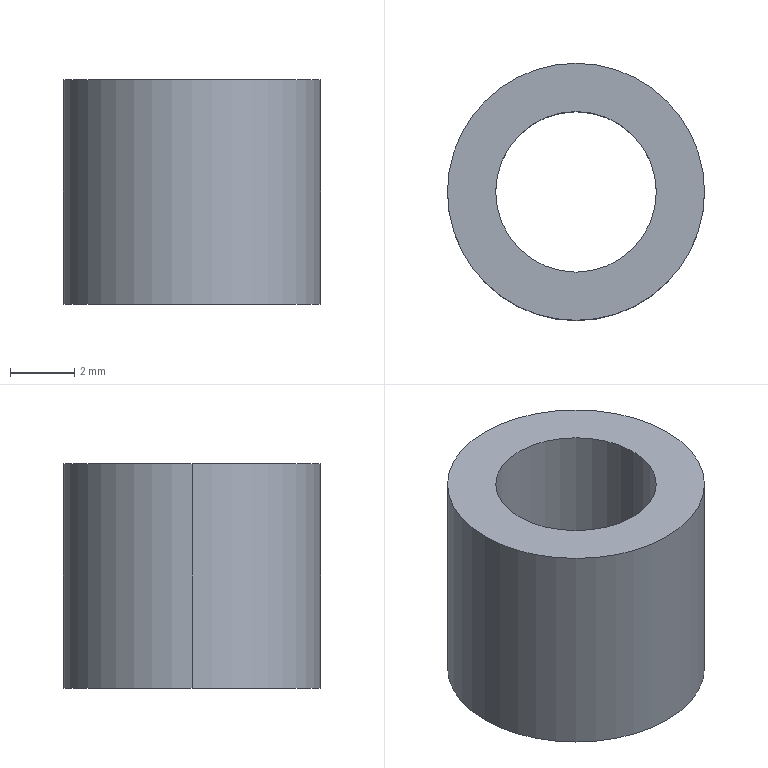Part | SolidWorks | features Extrusion 1 | 1 solid | 6 faces | box 8 x 8 x 7 mm | volume 214.414 mm3 | cylinder 4 | plane 2 | commonest cylinder face diameters 5 x2 8 x2
STEP:
#1=CARTESIAN_POINT('',(-2.5,0.,7.));
#2=VERTEX_POINT('',#1);
#3=CARTESIAN_POINT('',(2.5,0.,7.));
#4=VERTEX_POINT('',#3);
#5=CARTESIAN_POINT('',(0.,0.,7.));
#6=DIRECTION('',(0.,0.,1.));
#7=DIRECTION('',(1.,0.,0.));
#8=AXIS2_PLACEMENT_3D('',#5,#6,#7);
#9=CIRCLE('',#8,2.5);
#10=EDGE_CURVE('',#2,#4,#9,.T.);
#11=ORIENTED_EDGE('',*,*,#10,.T.);
#12=CARTESIAN_POINT('',(2.5,0.,0.));
#13=VERTEX_POINT('',#12);
#14=CARTESIAN_POINT('',(2.5,0.,7.));
#15=DIRECTION('',(0.,0.,-1.));
#16=VECTOR('',#15,1000.);
#17=LINE('',#14,#16);
#18=EDGE_CURVE('',#4,#13,#17,.T.);
#19=ORIENTED_EDGE('',*,*,#18,.T.);
#20=CARTESIAN_POINT('',(-2.5,0.,0.));
#21=VERTEX_POINT('',#20);
#22=CARTESIAN_POINT('',(0.,0.,0.));
#23=DIRECTION('',(0.,0.,1.));
#24=DIRECTION('',(1.,0.,0.));
#25=AXIS2_PLACEMENT_3D('',#22,#23,#24);
#26=CIRCLE('',#25,2.5);
#27=EDGE_CURVE('',#21,#13,#26,.T.);
#28=ORIENTED_EDGE('',*,*,#27,.F.);
#29=CARTESIAN_POINT('',(-2.5,0.,7.));
#30=DIRECTION('',(0.,0.,-1.));
#31=VECTOR('',#30,1000.);
#32=LINE('',#29,#31);
#33=EDGE_CURVE('',#2,#21,#32,.T.);
#34=ORIENTED_EDGE('',*,*,#33,.F.);
#35=EDGE_LOOP('',(#11,#19,#28,#34));
#36=FACE_OUTER_BOUND('',#35,.T.);
#37=CARTESIAN_POINT('',(0.,0.,7.));
#38=DIRECTION('',(0.,0.,-1.));
#39=DIRECTION('',(-1.,0.,0.));
#40=AXIS2_PLACEMENT_3D('',#37,#38,#39);
#41=CYLINDRICAL_SURFACE('',#40,2.5);
#42=ADVANCED_FACE('',(#36),#41,.F.);
#43=CARTESIAN_POINT('',(4.,0.,7.));
#44=VERTEX_POINT('',#43);
#45=CARTESIAN_POINT('',(-4.,0.,7.));
#46=VERTEX_POINT('',#45);
#47=CARTESIAN_POINT('',(0.,0.,7.));
#48=DIRECTION('',(0.,0.,1.));
#49=DIRECTION('',(1.,0.,0.));
#50=AXIS2_PLACEMENT_3D('',#47,#48,#49);
#51=CIRCLE('',#50,4.);
#52=EDGE_CURVE('',#44,#46,#51,.T.);
#53=ORIENTED_EDGE('',*,*,#52,.F.);
#54=CARTESIAN_POINT('',(4.,0.,0.));
#55=VERTEX_POINT('',#54);
#56=CARTESIAN_POINT('',(4.,0.,7.));
#57=DIRECTION('',(0.,0.,-1.));
#58=VECTOR('',#57,1000.);
#59=LINE('',#56,#58);
#60=EDGE_CURVE('',#44,#55,#59,.T.);
#61=ORIENTED_EDGE('',*,*,#60,.T.);
#62=CARTESIAN_POINT('',(-4.,0.,0.));
#63=VERTEX_POINT('',#62);
#64=CARTESIAN_POINT('',(0.,0.,0.));
#65=DIRECTION('',(0.,0.,1.));
#66=DIRECTION('',(1.,0.,0.));
#67=AXIS2_PLACEMENT_3D('',#64,#65,#66);
#68=CIRCLE('',#67,4.);
#69=EDGE_CURVE('',#55,#63,#68,.T.);
#70=ORIENTED_EDGE('',*,*,#69,.T.);
#71=CARTESIAN_POINT('',(-4.,0.,7.));
#72=DIRECTION('',(0.,0.,-1.));
#73=VECTOR('',#72,1000.);
#74=LINE('',#71,#73);
#75=EDGE_CURVE('',#46,#63,#74,.T.);
#76=ORIENTED_EDGE('',*,*,#75,.F.);
#77=EDGE_LOOP('',(#53,#61,#70,#76));
#78=FACE_OUTER_BOUND('',#77,.T.);
#79=CARTESIAN_POINT('',(0.,0.,7.));
#80=DIRECTION('',(0.,0.,-1.));
#81=DIRECTION('',(-1.,0.,0.));
#82=AXIS2_PLACEMENT_3D('',#79,#80,#81);
#83=CYLINDRICAL_SURFACE('',#82,4.);
#84=ADVANCED_FACE('',(#78),#83,.T.);
#85=CARTESIAN_POINT('',(0.,0.,7.));
#86=DIRECTION('',(0.,0.,1.));
#87=DIRECTION('',(1.,0.,0.));
#88=AXIS2_PLACEMENT_3D('',#85,#86,#87);
#89=CIRCLE('',#88,4.);
#90=EDGE_CURVE('',#46,#44,#89,.T.);
#91=ORIENTED_EDGE('',*,*,#90,.T.);
#92=ORIENTED_EDGE('',*,*,#52,.T.);
#93=EDGE_LOOP('',(#91,#92));
#94=FACE_OUTER_BOUND('',#93,.T.);
#95=ORIENTED_EDGE('',*,*,#10,.F.);
#96=CARTESIAN_POINT('',(0.,0.,7.));
#97=DIRECTION('',(0.,0.,1.));
#98=DIRECTION('',(1.,0.,0.));
#99=AXIS2_PLACEMENT_3D('',#96,#97,#98);
#100=CIRCLE('',#99,2.5);
#101=EDGE_CURVE('',#4,#2,#100,.T.);
#102=ORIENTED_EDGE('',*,*,#101,.F.);
#103=EDGE_LOOP('',(#95,#102));
#104=FACE_BOUND('',#103,.T.);
#105=CARTESIAN_POINT('',(0.,0.,7.));
#106=DIRECTION('',(0.,0.,1.));
#107=DIRECTION('',(1.,0.,0.));
#108=AXIS2_PLACEMENT_3D('',#105,#106,#107);
#109=PLANE('',#108);
#110=ADVANCED_FACE('',(#94,#104),#109,.T.);
#111=CARTESIAN_POINT('',(0.,0.,0.));
#112=DIRECTION('',(0.,0.,1.));
#113=DIRECTION('',(1.,0.,0.));
#114=AXIS2_PLACEMENT_3D('',#111,#112,#113);
#115=CIRCLE('',#114,4.);
#116=EDGE_CURVE('',#63,#55,#115,.T.);
#117=ORIENTED_EDGE('',*,*,#116,.F.);
#118=ORIENTED_EDGE('',*,*,#69,.F.);
#119=EDGE_LOOP('',(#117,#118));
#120=FACE_OUTER_BOUND('',#119,.T.);
#121=ORIENTED_EDGE('',*,*,#27,.T.);
#122=CARTESIAN_POINT('',(0.,0.,0.));
#123=DIRECTION('',(0.,0.,1.));
#124=DIRECTION('',(1.,0.,0.));
#125=AXIS2_PLACEMENT_3D('',#122,#123,#124);
#126=CIRCLE('',#125,2.5);
#127=EDGE_CURVE('',#13,#21,#126,.T.);
#128=ORIENTED_EDGE('',*,*,#127,.T.);
#129=EDGE_LOOP('',(#121,#128));
#130=FACE_BOUND('',#129,.T.);
#131=CARTESIAN_POINT('',(0.,0.,0.));
#132=DIRECTION('',(0.,0.,1.));
#133=DIRECTION('',(1.,0.,0.));
#134=AXIS2_PLACEMENT_3D('',#131,#132,#133);
#135=PLANE('',#134);
#136=ADVANCED_FACE('',(#120,#130),#135,.F.);
#137=ORIENTED_EDGE('',*,*,#60,.F.);
#138=ORIENTED_EDGE('',*,*,#90,.F.);
#139=ORIENTED_EDGE('',*,*,#75,.T.);
#140=ORIENTED_EDGE('',*,*,#116,.T.);
#141=EDGE_LOOP('',(#137,#138,#139,#140));
#142=FACE_OUTER_BOUND('',#141,.T.);
#143=CARTESIAN_POINT('',(0.,0.,7.));
#144=DIRECTION('',(0.,0.,-1.));
#145=DIRECTION('',(-1.,0.,0.));
#146=AXIS2_PLACEMENT_3D('',#143,#144,#145);
#147=CYLINDRICAL_SURFACE('',#146,4.);
#148=ADVANCED_FACE('',(#142),#147,.T.);
#149=ORIENTED_EDGE('',*,*,#18,.F.);
#150=ORIENTED_EDGE('',*,*,#101,.T.);
#151=ORIENTED_EDGE('',*,*,#33,.T.);
#152=ORIENTED_EDGE('',*,*,#127,.F.);
#153=EDGE_LOOP('',(#149,#150,#151,#152));
#154=FACE_OUTER_BOUND('',#153,.T.);
#155=CARTESIAN_POINT('',(0.,0.,7.));
#156=DIRECTION('',(0.,0.,-1.));
#157=DIRECTION('',(-1.,0.,0.));
#158=AXIS2_PLACEMENT_3D('',#155,#156,#157);
#159=CYLINDRICAL_SURFACE('',#158,2.5);
#160=ADVANCED_FACE('',(#154),#159,.F.);
#161=CLOSED_SHELL('',(#42,#84,#110,#136,#148,#160));
#162=MANIFOLD_SOLID_BREP('',#161);
#163=CARTESIAN_POINT('',(0.,0.,0.));
#164=DIRECTION('',(0.,0.,1.));
#165=DIRECTION('',(1.,0.,0.));
#166=AXIS2_PLACEMENT_3D('',#163,#164,#165);
#167=(LENGTH_UNIT()NAMED_UNIT(*)SI_UNIT(.MILLI.,.METRE.));
#168=UNCERTAINTY_MEASURE_WITH_UNIT(LENGTH_MEASURE(0.00001),#167,'','');
#169=(NAMED_UNIT(*)PLANE_ANGLE_UNIT()SI_UNIT($,.RADIAN.));
#170=(NAMED_UNIT(*)SI_UNIT($,.STERADIAN.)SOLID_ANGLE_UNIT());
#171=(GEOMETRIC_REPRESENTATION_CONTEXT(3)GLOBAL_UNCERTAINTY_ASSIGNED_CONTEXT((#168))GLOBAL_UNIT_ASSIGNED_CONTEXT((#167,#169,#170))REPRESENTATION_CONTEXT('',''));
#172=ADVANCED_BREP_SHAPE_REPRESENTATION('',(#162,#166),#171);